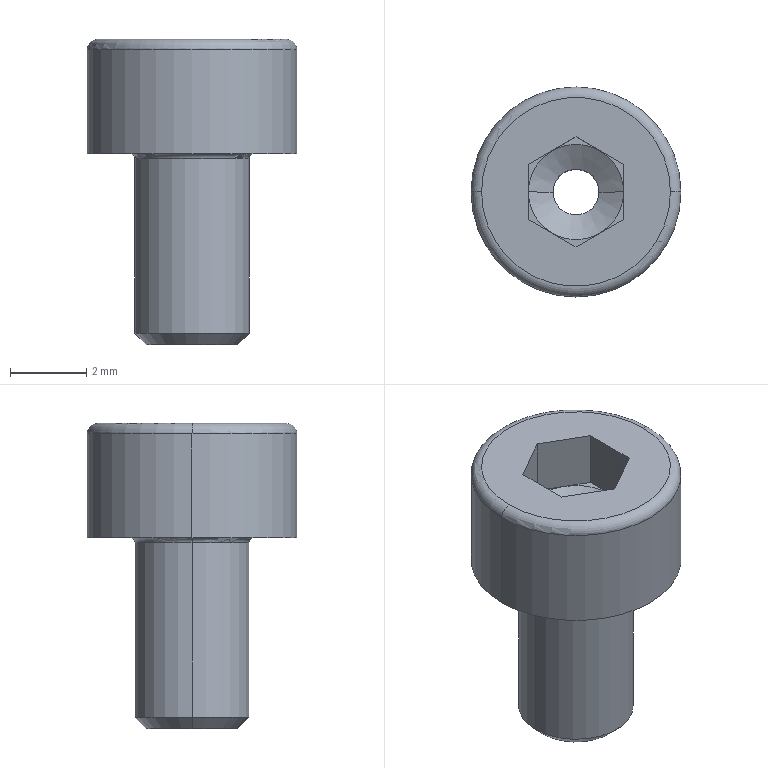Part | SolidWorks | features Fillet 2, ICE 2, Chamfer 1, Revolution 1 | 1 solid | 29 faces | box 5.5 x 5.5 x 8 mm | volume 89.884 mm3 | plane 15 | cylinder 6 | torus 4 | cone 4 | commonest cylinder face diameters 1.2 x2 3 x2 5.5 x2
STEP:
#1=CARTESIAN_POINT('',(-1.625,0.,0.));
#2=VERTEX_POINT('',#1);
#3=CARTESIAN_POINT('',(1.625,0.,0.));
#4=VERTEX_POINT('',#3);
#5=CARTESIAN_POINT('',(0.,0.,0.));
#6=DIRECTION('',(0.,0.,1.));
#7=DIRECTION('',(1.,0.,0.));
#8=AXIS2_PLACEMENT_3D('',#5,#6,#7);
#9=CIRCLE('',#8,1.625);
#10=EDGE_CURVE('',#2,#4,#9,.T.);
#11=ORIENTED_EDGE('',*,*,#10,.F.);
#12=CARTESIAN_POINT('',(-1.5,0.,-0.125));
#13=VERTEX_POINT('',#12);
#14=CARTESIAN_POINT('',(-1.625,0.,-0.125));
#15=DIRECTION('',(0.,1.,0.));
#16=DIRECTION('',(-1.,0.,0.));
#17=AXIS2_PLACEMENT_3D('',#14,#15,#16);
#18=CIRCLE('',#17,0.125);
#19=EDGE_CURVE('',#2,#13,#18,.T.);
#20=ORIENTED_EDGE('',*,*,#19,.T.);
#21=CARTESIAN_POINT('',(1.5,0.,-0.125));
#22=VERTEX_POINT('',#21);
#23=CARTESIAN_POINT('',(0.,0.,-0.125));
#24=DIRECTION('',(0.,0.,-1.));
#25=DIRECTION('',(1.,0.,0.));
#26=AXIS2_PLACEMENT_3D('',#23,#24,#25);
#27=CIRCLE('',#26,1.5);
#28=EDGE_CURVE('',#22,#13,#27,.T.);
#29=ORIENTED_EDGE('',*,*,#28,.F.);
#30=CARTESIAN_POINT('',(1.625,0.,-0.125));
#31=DIRECTION('',(0.,-1.,0.));
#32=DIRECTION('',(0.,0.,-1.));
#33=AXIS2_PLACEMENT_3D('',#30,#31,#32);
#34=CIRCLE('',#33,0.125);
#35=EDGE_CURVE('',#4,#22,#34,.T.);
#36=ORIENTED_EDGE('',*,*,#35,.F.);
#37=EDGE_LOOP('',(#11,#20,#29,#36));
#38=FACE_OUTER_BOUND('',#37,.T.);
#39=CARTESIAN_POINT('',(0.,0.,-0.125));
#40=DIRECTION('',(0.,0.,1.));
#41=DIRECTION('',(1.,0.,0.));
#42=AXIS2_PLACEMENT_3D('',#39,#40,#41);
#43=TOROIDAL_SURFACE('',#42,1.625,0.125);
#44=ADVANCED_FACE('',(#38),#43,.F.);
#45=CARTESIAN_POINT('',(-0.6,0.,1.125));
#46=VERTEX_POINT('',#45);
#47=CARTESIAN_POINT('',(0.6,0.,1.125));
#48=VERTEX_POINT('',#47);
#49=CARTESIAN_POINT('',(0.,0.,1.125));
#50=DIRECTION('',(0.,0.,1.));
#51=DIRECTION('',(1.,0.,0.));
#52=AXIS2_PLACEMENT_3D('',#49,#50,#51);
#53=CIRCLE('',#52,0.6);
#54=EDGE_CURVE('',#46,#48,#53,.T.);
#55=ORIENTED_EDGE('',*,*,#54,.F.);
#56=CARTESIAN_POINT('',(-1.25,0.,1.5));
#57=VERTEX_POINT('',#56);
#58=CARTESIAN_POINT('',(-1.25,0.,1.5));
#59=DIRECTION('',(-0.866,0.,0.5));
#60=VECTOR('',#59,1000.);
#61=LINE('',#58,#60);
#62=EDGE_CURVE('',#46,#57,#61,.T.);
#63=ORIENTED_EDGE('',*,*,#62,.T.);
#64=CARTESIAN_POINT('',(-0.625,-1.083,1.5));
#65=VERTEX_POINT('',#64);
#66=CARTESIAN_POINT('',(0.,0.,1.5));
#67=DIRECTION('',(0.,0.,1.));
#68=DIRECTION('',(1.,0.,0.));
#69=AXIS2_PLACEMENT_3D('',#66,#67,#68);
#70=CIRCLE('',#69,1.25);
#71=EDGE_CURVE('',#57,#65,#70,.T.);
#72=ORIENTED_EDGE('',*,*,#71,.T.);
#73=CARTESIAN_POINT('',(0.625,-1.083,1.5));
#74=VERTEX_POINT('',#73);
#75=CARTESIAN_POINT('',(0.,0.,1.5));
#76=DIRECTION('',(0.,0.,1.));
#77=DIRECTION('',(1.,0.,0.));
#78=AXIS2_PLACEMENT_3D('',#75,#76,#77);
#79=CIRCLE('',#78,1.25);
#80=EDGE_CURVE('',#65,#74,#79,.T.);
#81=ORIENTED_EDGE('',*,*,#80,.T.);
#82=CARTESIAN_POINT('',(1.25,0.,1.5));
#83=VERTEX_POINT('',#82);
#84=CARTESIAN_POINT('',(0.,0.,1.5));
#85=DIRECTION('',(0.,0.,1.));
#86=DIRECTION('',(1.,0.,0.));
#87=AXIS2_PLACEMENT_3D('',#84,#85,#86);
#88=CIRCLE('',#87,1.25);
#89=EDGE_CURVE('',#74,#83,#88,.T.);
#90=ORIENTED_EDGE('',*,*,#89,.T.);
#91=CARTESIAN_POINT('',(1.25,0.,1.5));
#92=DIRECTION('',(0.866,0.,0.5));
#93=VECTOR('',#92,1000.);
#94=LINE('',#91,#93);
#95=EDGE_CURVE('',#48,#83,#94,.T.);
#96=ORIENTED_EDGE('',*,*,#95,.F.);
#97=EDGE_LOOP('',(#55,#63,#72,#81,#90,#96));
#98=FACE_OUTER_BOUND('',#97,.T.);
#99=CARTESIAN_POINT('',(0.,0.,1.5));
#100=DIRECTION('',(0.,0.,1.));
#101=DIRECTION('',(1.,0.,0.));
#102=AXIS2_PLACEMENT_3D('',#99,#100,#101);
#103=CONICAL_SURFACE('',#102,1.25,1.047);
#104=ADVANCED_FACE('',(#98),#103,.F.);
#105=CARTESIAN_POINT('',(-1.2,0.,-5.));
#106=VERTEX_POINT('',#105);
#107=CARTESIAN_POINT('',(1.2,0.,-5.));
#108=VERTEX_POINT('',#107);
#109=CARTESIAN_POINT('',(0.,0.,-5.));
#110=DIRECTION('',(0.,0.,-1.));
#111=DIRECTION('',(1.,0.,0.));
#112=AXIS2_PLACEMENT_3D('',#109,#110,#111);
#113=CIRCLE('',#112,1.2);
#114=EDGE_CURVE('',#106,#108,#113,.T.);
#115=ORIENTED_EDGE('',*,*,#114,.F.);
#116=CARTESIAN_POINT('',(-1.5,0.,-4.7));
#117=VERTEX_POINT('',#116);
#118=CARTESIAN_POINT('',(-1.5,0.,-4.7));
#119=DIRECTION('',(-0.7071,0.,0.7071));
#120=VECTOR('',#119,1000.);
#121=LINE('',#118,#120);
#122=EDGE_CURVE('',#106,#117,#121,.T.);
#123=ORIENTED_EDGE('',*,*,#122,.T.);
#124=CARTESIAN_POINT('',(1.5,0.,-4.7));
#125=VERTEX_POINT('',#124);
#126=CARTESIAN_POINT('',(0.,0.,-4.7));
#127=DIRECTION('',(0.,0.,1.));
#128=DIRECTION('',(1.,0.,0.));
#129=AXIS2_PLACEMENT_3D('',#126,#127,#128);
#130=CIRCLE('',#129,1.5);
#131=EDGE_CURVE('',#125,#117,#130,.T.);
#132=ORIENTED_EDGE('',*,*,#131,.F.);
#133=CARTESIAN_POINT('',(1.5,0.,-4.7));
#134=DIRECTION('',(0.7071,0.,0.7071));
#135=VECTOR('',#134,1000.);
#136=LINE('',#133,#135);
#137=EDGE_CURVE('',#108,#125,#136,.T.);
#138=ORIENTED_EDGE('',*,*,#137,.F.);
#139=EDGE_LOOP('',(#115,#123,#132,#138));
#140=FACE_OUTER_BOUND('',#139,.T.);
#141=CARTESIAN_POINT('',(0.,0.,-4.7));
#142=DIRECTION('',(0.,0.,1.));
#143=DIRECTION('',(1.,0.,0.));
#144=AXIS2_PLACEMENT_3D('',#141,#142,#143);
#145=CONICAL_SURFACE('',#144,1.5,0.7854);
#146=ADVANCED_FACE('',(#140),#145,.T.);
#147=CARTESIAN_POINT('',(2.475,0.,3.));
#148=VERTEX_POINT('',#147);
#149=CARTESIAN_POINT('',(-2.475,0.,3.));
#150=VERTEX_POINT('',#149);
#151=CARTESIAN_POINT('',(0.,0.,3.));
#152=DIRECTION('',(0.,0.,1.));
#153=DIRECTION('',(-1.,0.,0.));
#154=AXIS2_PLACEMENT_3D('',#151,#152,#153);
#155=CIRCLE('',#154,2.475);
#156=EDGE_CURVE('',#148,#150,#155,.T.);
#157=ORIENTED_EDGE('',*,*,#156,.F.);
#158=CARTESIAN_POINT('',(2.75,0.,2.725));
#159=VERTEX_POINT('',#158);
#160=CARTESIAN_POINT('',(2.475,0.,2.725));
#161=DIRECTION('',(0.,1.,0.));
#162=DIRECTION('',(-1.,0.,0.));
#163=AXIS2_PLACEMENT_3D('',#160,#161,#162);
#164=CIRCLE('',#163,0.275);
#165=EDGE_CURVE('',#148,#159,#164,.T.);
#166=ORIENTED_EDGE('',*,*,#165,.T.);
#167=CARTESIAN_POINT('',(-2.75,0.,2.725));
#168=VERTEX_POINT('',#167);
#169=CARTESIAN_POINT('',(0.,0.,2.725));
#170=DIRECTION('',(0.,0.,-1.));
#171=DIRECTION('',(-1.,0.,0.));
#172=AXIS2_PLACEMENT_3D('',#169,#170,#171);
#173=CIRCLE('',#172,2.75);
#174=EDGE_CURVE('',#168,#159,#173,.T.);
#175=ORIENTED_EDGE('',*,*,#174,.F.);
#176=CARTESIAN_POINT('',(-2.475,0.,2.725));
#177=DIRECTION('',(0.,-1.,0.));
#178=DIRECTION('',(0.,0.,-1.));
#179=AXIS2_PLACEMENT_3D('',#176,#177,#178);
#180=CIRCLE('',#179,0.275);
#181=EDGE_CURVE('',#150,#168,#180,.T.);
#182=ORIENTED_EDGE('',*,*,#181,.F.);
#183=EDGE_LOOP('',(#157,#166,#175,#182));
#184=FACE_OUTER_BOUND('',#183,.T.);
#185=CARTESIAN_POINT('',(0.,0.,2.725));
#186=DIRECTION('',(0.,0.,-1.));
#187=DIRECTION('',(-1.,0.,0.));
#188=AXIS2_PLACEMENT_3D('',#185,#186,#187);
#189=TOROIDAL_SURFACE('',#188,2.475,0.275);
#190=ADVANCED_FACE('',(#184),#189,.T.);
#191=ORIENTED_EDGE('',*,*,#131,.T.);
#192=CARTESIAN_POINT('',(-1.5,0.,3.));
#193=DIRECTION('',(0.,0.,1.));
#194=VECTOR('',#193,1000.);
#195=LINE('',#192,#194);
#196=EDGE_CURVE('',#117,#13,#195,.T.);
#197=ORIENTED_EDGE('',*,*,#196,.T.);
#198=CARTESIAN_POINT('',(0.,0.,-0.125));
#199=DIRECTION('',(0.,0.,-1.));
#200=DIRECTION('',(1.,0.,0.));
#201=AXIS2_PLACEMENT_3D('',#198,#199,#200);
#202=CIRCLE('',#201,1.5);
#203=EDGE_CURVE('',#13,#22,#202,.T.);
#204=ORIENTED_EDGE('',*,*,#203,.T.);
#205=CARTESIAN_POINT('',(1.5,0.,3.));
#206=DIRECTION('',(0.,0.,1.));
#207=VECTOR('',#206,1000.);
#208=LINE('',#205,#207);
#209=EDGE_CURVE('',#125,#22,#208,.T.);
#210=ORIENTED_EDGE('',*,*,#209,.F.);
#211=EDGE_LOOP('',(#191,#197,#204,#210));
#212=FACE_OUTER_BOUND('',#211,.T.);
#213=CARTESIAN_POINT('',(0.,0.,3.));
#214=DIRECTION('',(0.,0.,1.));
#215=DIRECTION('',(1.,0.,0.));
#216=AXIS2_PLACEMENT_3D('',#213,#214,#215);
#217=CYLINDRICAL_SURFACE('',#216,1.5);
#218=ADVANCED_FACE('',(#212),#217,.T.);
#219=CARTESIAN_POINT('',(2.75,0.,0.));
#220=VERTEX_POINT('',#219);
#221=CARTESIAN_POINT('',(-2.75,0.,0.));
#222=VERTEX_POINT('',#221);
#223=CARTESIAN_POINT('',(0.,0.,0.));
#224=DIRECTION('',(0.,0.,1.));
#225=DIRECTION('',(1.,0.,0.));
#226=AXIS2_PLACEMENT_3D('',#223,#224,#225);
#227=CIRCLE('',#226,2.75);
#228=EDGE_CURVE('',#220,#222,#227,.T.);
#229=ORIENTED_EDGE('',*,*,#228,.T.);
#230=CARTESIAN_POINT('',(-2.75,0.,3.));
#231=DIRECTION('',(0.,0.,1.));
#232=VECTOR('',#231,1000.);
#233=LINE('',#230,#232);
#234=EDGE_CURVE('',#222,#168,#233,.T.);
#235=ORIENTED_EDGE('',*,*,#234,.T.);
#236=ORIENTED_EDGE('',*,*,#174,.T.);
#237=CARTESIAN_POINT('',(2.75,0.,3.));
#238=DIRECTION('',(0.,0.,1.));
#239=VECTOR('',#238,1000.);
#240=LINE('',#237,#239);
#241=EDGE_CURVE('',#220,#159,#240,.T.);
#242=ORIENTED_EDGE('',*,*,#241,.F.);
#243=EDGE_LOOP('',(#229,#235,#236,#242));
#244=FACE_OUTER_BOUND('',#243,.T.);
#245=CARTESIAN_POINT('',(0.,0.,3.));
#246=DIRECTION('',(0.,0.,1.));
#247=DIRECTION('',(1.,0.,0.));
#248=AXIS2_PLACEMENT_3D('',#245,#246,#247);
#249=CYLINDRICAL_SURFACE('',#248,2.75);
#250=ADVANCED_FACE('',(#244),#249,.T.);
#251=CARTESIAN_POINT('',(-0.6,0.,-5.));
#252=VERTEX_POINT('',#251);
#253=CARTESIAN_POINT('',(0.6,0.,-5.));
#254=VERTEX_POINT('',#253);
#255=CARTESIAN_POINT('',(0.,0.,-5.));
#256=DIRECTION('',(0.,0.,1.));
#257=DIRECTION('',(1.,0.,0.));
#258=AXIS2_PLACEMENT_3D('',#255,#256,#257);
#259=CIRCLE('',#258,0.6);
#260=EDGE_CURVE('',#252,#254,#259,.T.);
#261=ORIENTED_EDGE('',*,*,#260,.F.);
#262=CARTESIAN_POINT('',(-0.6,0.,3.));
#263=DIRECTION('',(0.,0.,1.));
#264=VECTOR('',#263,1000.);
#265=LINE('',#262,#264);
#266=EDGE_CURVE('',#252,#46,#265,.T.);
#267=ORIENTED_EDGE('',*,*,#266,.T.);
#268=ORIENTED_EDGE('',*,*,#54,.T.);
#269=CARTESIAN_POINT('',(0.6,0.,3.));
#270=DIRECTION('',(0.,0.,1.));
#271=VECTOR('',#270,1000.);
#272=LINE('',#269,#271);
#273=EDGE_CURVE('',#254,#48,#272,.T.);
#274=ORIENTED_EDGE('',*,*,#273,.F.);
#275=EDGE_LOOP('',(#261,#267,#268,#274));
#276=FACE_OUTER_BOUND('',#275,.T.);
#277=CARTESIAN_POINT('',(0.,0.,3.));
#278=DIRECTION('',(0.,0.,1.));
#279=DIRECTION('',(1.,0.,0.));
#280=AXIS2_PLACEMENT_3D('',#277,#278,#279);
#281=CYLINDRICAL_SURFACE('',#280,0.6);
#282=ADVANCED_FACE('',(#276),#281,.F.);
#283=CARTESIAN_POINT('',(0.625,1.083,1.5));
#284=VERTEX_POINT('',#283);
#285=CARTESIAN_POINT('',(0.,0.,1.5));
#286=DIRECTION('',(0.,0.,1.));
#287=DIRECTION('',(1.,0.,0.));
#288=AXIS2_PLACEMENT_3D('',#285,#286,#287);
#289=CIRCLE('',#288,1.25);
#290=EDGE_CURVE('',#83,#284,#289,.T.);
#291=ORIENTED_EDGE('',*,*,#290,.F.);
#292=CARTESIAN_POINT('',(1.25,0.7217,1.5));
#293=VERTEX_POINT('',#292);
#294=CARTESIAN_POINT('',(1.25,-0.7217,1.5));
#295=DIRECTION('',(0.,1.,0.));
#296=VECTOR('',#295,1000.);
#297=LINE('',#294,#296);
#298=EDGE_CURVE('',#83,#293,#297,.T.);
#299=ORIENTED_EDGE('',*,*,#298,.T.);
#300=CARTESIAN_POINT('',(1.25,0.7217,1.5));
#301=DIRECTION('',(-0.866,0.5,0.));
#302=VECTOR('',#301,1000.);
#303=LINE('',#300,#302);
#304=EDGE_CURVE('',#293,#284,#303,.T.);
#305=ORIENTED_EDGE('',*,*,#304,.T.);
#306=EDGE_LOOP('',(#291,#299,#305));
#307=FACE_OUTER_BOUND('',#306,.T.);
#308=CARTESIAN_POINT('',(0.,1.443,1.5));
#309=DIRECTION('',(0.,0.,1.));
#310=DIRECTION('',(1.,0.,0.));
#311=AXIS2_PLACEMENT_3D('',#308,#309,#310);
#312=PLANE('',#311);
#313=ADVANCED_FACE('',(#307),#312,.T.);
#314=CARTESIAN_POINT('',(-0.625,1.083,1.5));
#315=VERTEX_POINT('',#314);
#316=CARTESIAN_POINT('',(0.,0.,1.5));
#317=DIRECTION('',(0.,0.,1.));
#318=DIRECTION('',(1.,0.,0.));
#319=AXIS2_PLACEMENT_3D('',#316,#317,#318);
#320=CIRCLE('',#319,1.25);
#321=EDGE_CURVE('',#284,#315,#320,.T.);
#322=ORIENTED_EDGE('',*,*,#321,.F.);
#323=CARTESIAN_POINT('',(0.,1.443,1.5));
#324=VERTEX_POINT('',#323);
#325=CARTESIAN_POINT('',(1.25,0.7217,1.5));
#326=DIRECTION('',(-0.866,0.5,0.));
#327=VECTOR('',#326,1000.);
#328=LINE('',#325,#327);
#329=EDGE_CURVE('',#284,#324,#328,.T.);
#330=ORIENTED_EDGE('',*,*,#329,.T.);
#331=CARTESIAN_POINT('',(0.,1.443,1.5));
#332=DIRECTION('',(-0.866,-0.5,0.));
#333=VECTOR('',#332,1000.);
#334=LINE('',#331,#333);
#335=EDGE_CURVE('',#324,#315,#334,.T.);
#336=ORIENTED_EDGE('',*,*,#335,.T.);
#337=EDGE_LOOP('',(#322,#330,#336));
#338=FACE_OUTER_BOUND('',#337,.T.);
#339=CARTESIAN_POINT('',(0.,1.443,1.5));
#340=DIRECTION('',(0.,0.,1.));
#341=DIRECTION('',(1.,0.,0.));
#342=AXIS2_PLACEMENT_3D('',#339,#340,#341);
#343=PLANE('',#342);
#344=ADVANCED_FACE('',(#338),#343,.T.);
#345=CARTESIAN_POINT('',(0.,0.,1.5));
#346=DIRECTION('',(0.,0.,1.));
#347=DIRECTION('',(1.,0.,0.));
#348=AXIS2_PLACEMENT_3D('',#345,#346,#347);
#349=CIRCLE('',#348,1.25);
#350=EDGE_CURVE('',#315,#57,#349,.T.);
#351=ORIENTED_EDGE('',*,*,#350,.F.);
#352=CARTESIAN_POINT('',(-1.25,0.7217,1.5));
#353=VERTEX_POINT('',#352);
#354=CARTESIAN_POINT('',(0.,1.443,1.5));
#355=DIRECTION('',(-0.866,-0.5,0.));
#356=VECTOR('',#355,1000.);
#357=LINE('',#354,#356);
#358=EDGE_CURVE('',#315,#353,#357,.T.);
#359=ORIENTED_EDGE('',*,*,#358,.T.);
#360=CARTESIAN_POINT('',(-1.25,0.7217,1.5));
#361=DIRECTION('',(0.,-1.,0.));
#362=VECTOR('',#361,1000.);
#363=LINE('',#360,#362);
#364=EDGE_CURVE('',#353,#57,#363,.T.);
#365=ORIENTED_EDGE('',*,*,#364,.T.);
#366=EDGE_LOOP('',(#351,#359,#365));
#367=FACE_OUTER_BOUND('',#366,.T.);
#368=CARTESIAN_POINT('',(0.,1.443,1.5));
#369=DIRECTION('',(0.,0.,1.));
#370=DIRECTION('',(1.,0.,0.));
#371=AXIS2_PLACEMENT_3D('',#368,#369,#370);
#372=PLANE('',#371);
#373=ADVANCED_FACE('',(#367),#372,.T.);
#374=ORIENTED_EDGE('',*,*,#71,.F.);
#375=CARTESIAN_POINT('',(-1.25,-0.7217,1.5));
#376=VERTEX_POINT('',#375);
#377=CARTESIAN_POINT('',(-1.25,0.7217,1.5));
#378=DIRECTION('',(0.,-1.,0.));
#379=VECTOR('',#378,1000.);
#380=LINE('',#377,#379);
#381=EDGE_CURVE('',#57,#376,#380,.T.);
#382=ORIENTED_EDGE('',*,*,#381,.T.);
#383=CARTESIAN_POINT('',(-1.25,-0.7217,1.5));
#384=DIRECTION('',(0.866,-0.5,0.));
#385=VECTOR('',#384,1000.);
#386=LINE('',#383,#385);
#387=EDGE_CURVE('',#376,#65,#386,.T.);
#388=ORIENTED_EDGE('',*,*,#387,.T.);
#389=EDGE_LOOP('',(#374,#382,#388));
#390=FACE_OUTER_BOUND('',#389,.T.);
#391=CARTESIAN_POINT('',(0.,1.443,1.5));
#392=DIRECTION('',(0.,0.,1.));
#393=DIRECTION('',(1.,0.,0.));
#394=AXIS2_PLACEMENT_3D('',#391,#392,#393);
#395=PLANE('',#394);
#396=ADVANCED_FACE('',(#390),#395,.T.);
#397=ORIENTED_EDGE('',*,*,#80,.F.);
#398=CARTESIAN_POINT('',(0.,-1.443,1.5));
#399=VERTEX_POINT('',#398);
#400=CARTESIAN_POINT('',(-1.25,-0.7217,1.5));
#401=DIRECTION('',(0.866,-0.5,0.));
#402=VECTOR('',#401,1000.);
#403=LINE('',#400,#402);
#404=EDGE_CURVE('',#65,#399,#403,.T.);
#405=ORIENTED_EDGE('',*,*,#404,.T.);
#406=CARTESIAN_POINT('',(0.,-1.443,1.5));
#407=DIRECTION('',(0.866,0.5,0.));
#408=VECTOR('',#407,1000.);
#409=LINE('',#406,#408);
#410=EDGE_CURVE('',#399,#74,#409,.T.);
#411=ORIENTED_EDGE('',*,*,#410,.T.);
#412=EDGE_LOOP('',(#397,#405,#411));
#413=FACE_OUTER_BOUND('',#412,.T.);
#414=CARTESIAN_POINT('',(0.,1.443,1.5));
#415=DIRECTION('',(0.,0.,1.));
#416=DIRECTION('',(1.,0.,0.));
#417=AXIS2_PLACEMENT_3D('',#414,#415,#416);
#418=PLANE('',#417);
#419=ADVANCED_FACE('',(#413),#418,.T.);
#420=ORIENTED_EDGE('',*,*,#266,.F.);
#421=CARTESIAN_POINT('',(0.,0.,-5.));
#422=DIRECTION('',(0.,0.,1.));
#423=DIRECTION('',(1.,0.,0.));
#424=AXIS2_PLACEMENT_3D('',#421,#422,#423);
#425=CIRCLE('',#424,0.6);
#426=EDGE_CURVE('',#254,#252,#425,.T.);
#427=ORIENTED_EDGE('',*,*,#426,.F.);
#428=ORIENTED_EDGE('',*,*,#273,.T.);
#429=CARTESIAN_POINT('',(0.,0.,1.125));
#430=DIRECTION('',(0.,0.,1.));
#431=DIRECTION('',(1.,0.,0.));
#432=AXIS2_PLACEMENT_3D('',#429,#430,#431);
#433=CIRCLE('',#432,0.6);
#434=EDGE_CURVE('',#48,#46,#433,.T.);
#435=ORIENTED_EDGE('',*,*,#434,.T.);
#436=EDGE_LOOP('',(#420,#427,#428,#435));
#437=FACE_OUTER_BOUND('',#436,.T.);
#438=CARTESIAN_POINT('',(0.,0.,3.));
#439=DIRECTION('',(0.,0.,1.));
#440=DIRECTION('',(1.,0.,0.));
#441=AXIS2_PLACEMENT_3D('',#438,#439,#440);
#442=CYLINDRICAL_SURFACE('',#441,0.6);
#443=ADVANCED_FACE('',(#437),#442,.F.);
#444=ORIENTED_EDGE('',*,*,#234,.F.);
#445=CARTESIAN_POINT('',(0.,0.,0.));
#446=DIRECTION('',(0.,0.,1.));
#447=DIRECTION('',(1.,0.,0.));
#448=AXIS2_PLACEMENT_3D('',#445,#446,#447);
#449=CIRCLE('',#448,2.75);
#450=EDGE_CURVE('',#222,#220,#449,.T.);
#451=ORIENTED_EDGE('',*,*,#450,.T.);
#452=ORIENTED_EDGE('',*,*,#241,.T.);
#453=CARTESIAN_POINT('',(0.,0.,2.725));
#454=DIRECTION('',(0.,0.,-1.));
#455=DIRECTION('',(-1.,0.,0.));
#456=AXIS2_PLACEMENT_3D('',#453,#454,#455);
#457=CIRCLE('',#456,2.75);
#458=EDGE_CURVE('',#159,#168,#457,.T.);
#459=ORIENTED_EDGE('',*,*,#458,.T.);
#460=EDGE_LOOP('',(#444,#451,#452,#459));
#461=FACE_OUTER_BOUND('',#460,.T.);
#462=CARTESIAN_POINT('',(0.,0.,3.));
#463=DIRECTION('',(0.,0.,1.));
#464=DIRECTION('',(1.,0.,0.));
#465=AXIS2_PLACEMENT_3D('',#462,#463,#464);
#466=CYLINDRICAL_SURFACE('',#465,2.75);
#467=ADVANCED_FACE('',(#461),#466,.T.);
#468=CARTESIAN_POINT('',(0.,0.,0.));
#469=DIRECTION('',(0.,0.,1.));
#470=DIRECTION('',(1.,0.,0.));
#471=AXIS2_PLACEMENT_3D('',#468,#469,#470);
#472=CIRCLE('',#471,1.625);
#473=EDGE_CURVE('',#4,#2,#472,.T.);
#474=ORIENTED_EDGE('',*,*,#473,.T.);
#475=ORIENTED_EDGE('',*,*,#10,.T.);
#476=EDGE_LOOP('',(#474,#475));
#477=FACE_BOUND('',#476,.T.);
#478=ORIENTED_EDGE('',*,*,#228,.F.);
#479=ORIENTED_EDGE('',*,*,#450,.F.);
#480=EDGE_LOOP('',(#478,#479));
#481=FACE_OUTER_BOUND('',#480,.T.);
#482=CARTESIAN_POINT('',(0.,2.75,0.));
#483=DIRECTION('',(0.,0.,1.));
#484=DIRECTION('',(1.,0.,0.));
#485=AXIS2_PLACEMENT_3D('',#482,#483,#484);
#486=PLANE('',#485);
#487=ADVANCED_FACE('',(#477,#481),#486,.F.);
#488=ORIENTED_EDGE('',*,*,#196,.F.);
#489=CARTESIAN_POINT('',(0.,0.,-4.7));
#490=DIRECTION('',(0.,0.,1.));
#491=DIRECTION('',(1.,0.,0.));
#492=AXIS2_PLACEMENT_3D('',#489,#490,#491);
#493=CIRCLE('',#492,1.5);
#494=EDGE_CURVE('',#117,#125,#493,.T.);
#495=ORIENTED_EDGE('',*,*,#494,.T.);
#496=ORIENTED_EDGE('',*,*,#209,.T.);
#497=ORIENTED_EDGE('',*,*,#28,.T.);
#498=EDGE_LOOP('',(#488,#495,#496,#497));
#499=FACE_OUTER_BOUND('',#498,.T.);
#500=CARTESIAN_POINT('',(0.,0.,3.));
#501=DIRECTION('',(0.,0.,1.));
#502=DIRECTION('',(1.,0.,0.));
#503=AXIS2_PLACEMENT_3D('',#500,#501,#502);
#504=CYLINDRICAL_SURFACE('',#503,1.5);
#505=ADVANCED_FACE('',(#499),#504,.T.);
#506=CARTESIAN_POINT('',(0.,0.,-5.));
#507=DIRECTION('',(0.,0.,-1.));
#508=DIRECTION('',(1.,0.,0.));
#509=AXIS2_PLACEMENT_3D('',#506,#507,#508);
#510=CIRCLE('',#509,1.2);
#511=EDGE_CURVE('',#108,#106,#510,.T.);
#512=ORIENTED_EDGE('',*,*,#511,.T.);
#513=ORIENTED_EDGE('',*,*,#114,.T.);
#514=EDGE_LOOP('',(#512,#513));
#515=FACE_OUTER_BOUND('',#514,.T.);
#516=ORIENTED_EDGE('',*,*,#426,.T.);
#517=ORIENTED_EDGE('',*,*,#260,.T.);
#518=EDGE_LOOP('',(#516,#517));
#519=FACE_BOUND('',#518,.T.);
#520=CARTESIAN_POINT('',(0.,1.5,-5.));
#521=DIRECTION('',(0.,0.,1.));
#522=DIRECTION('',(1.,0.,0.));
#523=AXIS2_PLACEMENT_3D('',#520,#521,#522);
#524=PLANE('',#523);
#525=ADVANCED_FACE('',(#515,#519),#524,.F.);
#526=CARTESIAN_POINT('',(0.,0.,3.));
#527=DIRECTION('',(0.,0.,1.));
#528=DIRECTION('',(-1.,0.,0.));
#529=AXIS2_PLACEMENT_3D('',#526,#527,#528);
#530=CIRCLE('',#529,2.475);
#531=EDGE_CURVE('',#150,#148,#530,.T.);
#532=ORIENTED_EDGE('',*,*,#531,.T.);
#533=ORIENTED_EDGE('',*,*,#156,.T.);
#534=EDGE_LOOP('',(#532,#533));
#535=FACE_OUTER_BOUND('',#534,.T.);
#536=CARTESIAN_POINT('',(0.,1.443,3.));
#537=VERTEX_POINT('',#536);
#538=CARTESIAN_POINT('',(-1.25,0.7217,3.));
#539=VERTEX_POINT('',#538);
#540=CARTESIAN_POINT('',(0.,1.443,3.));
#541=DIRECTION('',(-0.866,-0.5,0.));
#542=VECTOR('',#541,1000.);
#543=LINE('',#540,#542);
#544=EDGE_CURVE('',#537,#539,#543,.T.);
#545=ORIENTED_EDGE('',*,*,#544,.F.);
#546=CARTESIAN_POINT('',(1.25,0.7217,3.));
#547=VERTEX_POINT('',#546);
#548=CARTESIAN_POINT('',(1.25,0.7217,3.));
#549=DIRECTION('',(-0.866,0.5,0.));
#550=VECTOR('',#549,1000.);
#551=LINE('',#548,#550);
#552=EDGE_CURVE('',#547,#537,#551,.T.);
#553=ORIENTED_EDGE('',*,*,#552,.F.);
#554=CARTESIAN_POINT('',(1.25,-0.7217,3.));
#555=VERTEX_POINT('',#554);
#556=CARTESIAN_POINT('',(1.25,-0.7217,3.));
#557=DIRECTION('',(0.,1.,0.));
#558=VECTOR('',#557,1000.);
#559=LINE('',#556,#558);
#560=EDGE_CURVE('',#555,#547,#559,.T.);
#561=ORIENTED_EDGE('',*,*,#560,.F.);
#562=CARTESIAN_POINT('',(0.,-1.443,3.));
#563=VERTEX_POINT('',#562);
#564=CARTESIAN_POINT('',(0.,-1.443,3.));
#565=DIRECTION('',(0.866,0.5,0.));
#566=VECTOR('',#565,1000.);
#567=LINE('',#564,#566);
#568=EDGE_CURVE('',#563,#555,#567,.T.);
#569=ORIENTED_EDGE('',*,*,#568,.F.);
#570=CARTESIAN_POINT('',(-1.25,-0.7217,3.));
#571=VERTEX_POINT('',#570);
#572=CARTESIAN_POINT('',(-1.25,-0.7217,3.));
#573=DIRECTION('',(0.866,-0.5,0.));
#574=VECTOR('',#573,1000.);
#575=LINE('',#572,#574);
#576=EDGE_CURVE('',#571,#563,#575,.T.);
#577=ORIENTED_EDGE('',*,*,#576,.F.);
#578=CARTESIAN_POINT('',(-1.25,0.7217,3.));
#579=DIRECTION('',(0.,-1.,0.));
#580=VECTOR('',#579,1000.);
#581=LINE('',#578,#580);
#582=EDGE_CURVE('',#539,#571,#581,.T.);
#583=ORIENTED_EDGE('',*,*,#582,.F.);
#584=EDGE_LOOP('',(#545,#553,#561,#569,#577,#583));
#585=FACE_BOUND('',#584,.T.);
#586=CARTESIAN_POINT('',(0.,0.6,3.));
#587=DIRECTION('',(0.,0.,-1.));
#588=DIRECTION('',(-1.,0.,0.));
#589=AXIS2_PLACEMENT_3D('',#586,#587,#588);
#590=PLANE('',#589);
#591=ADVANCED_FACE('',(#535,#585),#590,.F.);
#592=ORIENTED_EDGE('',*,*,#89,.F.);
#593=CARTESIAN_POINT('',(1.25,-0.7217,1.5));
#594=VERTEX_POINT('',#593);
#595=CARTESIAN_POINT('',(0.,-1.443,1.5));
#596=DIRECTION('',(0.866,0.5,0.));
#597=VECTOR('',#596,1000.);
#598=LINE('',#595,#597);
#599=EDGE_CURVE('',#74,#594,#598,.T.);
#600=ORIENTED_EDGE('',*,*,#599,.T.);
#601=CARTESIAN_POINT('',(1.25,-0.7217,1.5));
#602=DIRECTION('',(0.,1.,0.));
#603=VECTOR('',#602,1000.);
#604=LINE('',#601,#603);
#605=EDGE_CURVE('',#594,#83,#604,.T.);
#606=ORIENTED_EDGE('',*,*,#605,.T.);
#607=EDGE_LOOP('',(#592,#600,#606));
#608=FACE_OUTER_BOUND('',#607,.T.);
#609=CARTESIAN_POINT('',(0.,1.443,1.5));
#610=DIRECTION('',(0.,0.,1.));
#611=DIRECTION('',(1.,0.,0.));
#612=AXIS2_PLACEMENT_3D('',#609,#610,#611);
#613=PLANE('',#612);
#614=ADVANCED_FACE('',(#608),#613,.T.);
#615=ORIENTED_EDGE('',*,*,#552,.T.);
#616=CARTESIAN_POINT('',(0.,1.443,1.5));
#617=DIRECTION('',(0.,0.,1.));
#618=VECTOR('',#617,1000.);
#619=LINE('',#616,#618);
#620=EDGE_CURVE('',#324,#537,#619,.T.);
#621=ORIENTED_EDGE('',*,*,#620,.F.);
#622=ORIENTED_EDGE('',*,*,#329,.F.);
#623=ORIENTED_EDGE('',*,*,#304,.F.);
#624=CARTESIAN_POINT('',(1.25,0.7217,1.5));
#625=DIRECTION('',(0.,0.,1.));
#626=VECTOR('',#625,1000.);
#627=LINE('',#624,#626);
#628=EDGE_CURVE('',#293,#547,#627,.T.);
#629=ORIENTED_EDGE('',*,*,#628,.T.);
#630=EDGE_LOOP('',(#615,#621,#622,#623,#629));
#631=FACE_OUTER_BOUND('',#630,.T.);
#632=CARTESIAN_POINT('',(1.25,0.7217,1.5));
#633=DIRECTION('',(0.5,0.866,0.));
#634=DIRECTION('',(-0.866,0.5,0.));
#635=AXIS2_PLACEMENT_3D('',#632,#633,#634);
#636=PLANE('',#635);
#637=ADVANCED_FACE('',(#631),#636,.F.);
#638=ORIENTED_EDGE('',*,*,#560,.T.);
#639=ORIENTED_EDGE('',*,*,#628,.F.);
#640=ORIENTED_EDGE('',*,*,#298,.F.);
#641=ORIENTED_EDGE('',*,*,#605,.F.);
#642=CARTESIAN_POINT('',(1.25,-0.7217,1.5));
#643=DIRECTION('',(0.,0.,1.));
#644=VECTOR('',#643,1000.);
#645=LINE('',#642,#644);
#646=EDGE_CURVE('',#594,#555,#645,.T.);
#647=ORIENTED_EDGE('',*,*,#646,.T.);
#648=EDGE_LOOP('',(#638,#639,#640,#641,#647));
#649=FACE_OUTER_BOUND('',#648,.T.);
#650=CARTESIAN_POINT('',(1.25,-0.7217,1.5));
#651=DIRECTION('',(1.,0.,0.));
#652=DIRECTION('',(0.,0.,-1.));
#653=AXIS2_PLACEMENT_3D('',#650,#651,#652);
#654=PLANE('',#653);
#655=ADVANCED_FACE('',(#649),#654,.F.);
#656=ORIENTED_EDGE('',*,*,#568,.T.);
#657=ORIENTED_EDGE('',*,*,#646,.F.);
#658=ORIENTED_EDGE('',*,*,#599,.F.);
#659=ORIENTED_EDGE('',*,*,#410,.F.);
#660=CARTESIAN_POINT('',(0.,-1.443,1.5));
#661=DIRECTION('',(0.,0.,1.));
#662=VECTOR('',#661,1000.);
#663=LINE('',#660,#662);
#664=EDGE_CURVE('',#399,#563,#663,.T.);
#665=ORIENTED_EDGE('',*,*,#664,.T.);
#666=EDGE_LOOP('',(#656,#657,#658,#659,#665));
#667=FACE_OUTER_BOUND('',#666,.T.);
#668=CARTESIAN_POINT('',(0.,-1.443,1.5));
#669=DIRECTION('',(0.5,-0.866,0.));
#670=DIRECTION('',(0.866,0.5,0.));
#671=AXIS2_PLACEMENT_3D('',#668,#669,#670);
#672=PLANE('',#671);
#673=ADVANCED_FACE('',(#667),#672,.F.);
#674=ORIENTED_EDGE('',*,*,#576,.T.);
#675=ORIENTED_EDGE('',*,*,#664,.F.);
#676=ORIENTED_EDGE('',*,*,#404,.F.);
#677=ORIENTED_EDGE('',*,*,#387,.F.);
#678=CARTESIAN_POINT('',(-1.25,-0.7217,1.5));
#679=DIRECTION('',(0.,0.,1.));
#680=VECTOR('',#679,1000.);
#681=LINE('',#678,#680);
#682=EDGE_CURVE('',#376,#571,#681,.T.);
#683=ORIENTED_EDGE('',*,*,#682,.T.);
#684=EDGE_LOOP('',(#674,#675,#676,#677,#683));
#685=FACE_OUTER_BOUND('',#684,.T.);
#686=CARTESIAN_POINT('',(-1.25,-0.7217,1.5));
#687=DIRECTION('',(-0.5,-0.866,0.));
#688=DIRECTION('',(0.866,-0.5,0.));
#689=AXIS2_PLACEMENT_3D('',#686,#687,#688);
#690=PLANE('',#689);
#691=ADVANCED_FACE('',(#685),#690,.F.);
#692=ORIENTED_EDGE('',*,*,#582,.T.);
#693=ORIENTED_EDGE('',*,*,#682,.F.);
#694=ORIENTED_EDGE('',*,*,#381,.F.);
#695=ORIENTED_EDGE('',*,*,#364,.F.);
#696=CARTESIAN_POINT('',(-1.25,0.7217,1.5));
#697=DIRECTION('',(0.,0.,1.));
#698=VECTOR('',#697,1000.);
#699=LINE('',#696,#698);
#700=EDGE_CURVE('',#353,#539,#699,.T.);
#701=ORIENTED_EDGE('',*,*,#700,.T.);
#702=EDGE_LOOP('',(#692,#693,#694,#695,#701));
#703=FACE_OUTER_BOUND('',#702,.T.);
#704=CARTESIAN_POINT('',(-1.25,0.7217,1.5));
#705=DIRECTION('',(-1.,0.,0.));
#706=DIRECTION('',(0.,-1.,0.));
#707=AXIS2_PLACEMENT_3D('',#704,#705,#706);
#708=PLANE('',#707);
#709=ADVANCED_FACE('',(#703),#708,.F.);
#710=ORIENTED_EDGE('',*,*,#544,.T.);
#711=ORIENTED_EDGE('',*,*,#700,.F.);
#712=ORIENTED_EDGE('',*,*,#358,.F.);
#713=ORIENTED_EDGE('',*,*,#335,.F.);
#714=ORIENTED_EDGE('',*,*,#620,.T.);
#715=EDGE_LOOP('',(#710,#711,#712,#713,#714));
#716=FACE_OUTER_BOUND('',#715,.T.);
#717=CARTESIAN_POINT('',(0.,1.443,1.5));
#718=DIRECTION('',(-0.5,0.866,0.));
#719=DIRECTION('',(-0.866,-0.5,0.));
#720=AXIS2_PLACEMENT_3D('',#717,#718,#719);
#721=PLANE('',#720);
#722=ADVANCED_FACE('',(#716),#721,.F.);
#723=ORIENTED_EDGE('',*,*,#165,.F.);
#724=ORIENTED_EDGE('',*,*,#531,.F.);
#725=ORIENTED_EDGE('',*,*,#181,.T.);
#726=ORIENTED_EDGE('',*,*,#458,.F.);
#727=EDGE_LOOP('',(#723,#724,#725,#726));
#728=FACE_OUTER_BOUND('',#727,.T.);
#729=CARTESIAN_POINT('',(0.,0.,2.725));
#730=DIRECTION('',(0.,0.,-1.));
#731=DIRECTION('',(-1.,0.,0.));
#732=AXIS2_PLACEMENT_3D('',#729,#730,#731);
#733=TOROIDAL_SURFACE('',#732,2.475,0.275);
#734=ADVANCED_FACE('',(#728),#733,.T.);
#735=ORIENTED_EDGE('',*,*,#122,.F.);
#736=ORIENTED_EDGE('',*,*,#511,.F.);
#737=ORIENTED_EDGE('',*,*,#137,.T.);
#738=ORIENTED_EDGE('',*,*,#494,.F.);
#739=EDGE_LOOP('',(#735,#736,#737,#738));
#740=FACE_OUTER_BOUND('',#739,.T.);
#741=CARTESIAN_POINT('',(0.,0.,-4.7));
#742=DIRECTION('',(0.,0.,1.));
#743=DIRECTION('',(1.,0.,0.));
#744=AXIS2_PLACEMENT_3D('',#741,#742,#743);
#745=CONICAL_SURFACE('',#744,1.5,0.7854);
#746=ADVANCED_FACE('',(#740),#745,.T.);
#747=ORIENTED_EDGE('',*,*,#62,.F.);
#748=ORIENTED_EDGE('',*,*,#434,.F.);
#749=ORIENTED_EDGE('',*,*,#95,.T.);
#750=ORIENTED_EDGE('',*,*,#290,.T.);
#751=ORIENTED_EDGE('',*,*,#321,.T.);
#752=ORIENTED_EDGE('',*,*,#350,.T.);
#753=EDGE_LOOP('',(#747,#748,#749,#750,#751,#752));
#754=FACE_OUTER_BOUND('',#753,.T.);
#755=CARTESIAN_POINT('',(0.,0.,1.5));
#756=DIRECTION('',(0.,0.,1.));
#757=DIRECTION('',(1.,0.,0.));
#758=AXIS2_PLACEMENT_3D('',#755,#756,#757);
#759=CONICAL_SURFACE('',#758,1.25,1.047);
#760=ADVANCED_FACE('',(#754),#759,.F.);
#761=ORIENTED_EDGE('',*,*,#19,.F.);
#762=ORIENTED_EDGE('',*,*,#473,.F.);
#763=ORIENTED_EDGE('',*,*,#35,.T.);
#764=ORIENTED_EDGE('',*,*,#203,.F.);
#765=EDGE_LOOP('',(#761,#762,#763,#764));
#766=FACE_OUTER_BOUND('',#765,.T.);
#767=CARTESIAN_POINT('',(0.,0.,-0.125));
#768=DIRECTION('',(0.,0.,1.));
#769=DIRECTION('',(1.,0.,0.));
#770=AXIS2_PLACEMENT_3D('',#767,#768,#769);
#771=TOROIDAL_SURFACE('',#770,1.625,0.125);
#772=ADVANCED_FACE('',(#766),#771,.F.);
#773=CLOSED_SHELL('',(#44,#104,#146,#190,#218,#250,#282,#313,#344,#373,#396,#419,#443,#467,#487,#505,#525,#591,#614,#637,#655,#673,#691,#709,#722,#734,#746,#760,#772));
#774=MANIFOLD_SOLID_BREP('',#773);
#775=CARTESIAN_POINT('',(0.,0.,0.));
#776=DIRECTION('',(0.,0.,1.));
#777=DIRECTION('',(1.,0.,0.));
#778=AXIS2_PLACEMENT_3D('',#775,#776,#777);
#779=(LENGTH_UNIT()NAMED_UNIT(*)SI_UNIT(.MILLI.,.METRE.));
#780=UNCERTAINTY_MEASURE_WITH_UNIT(LENGTH_MEASURE(0.00001),#779,'','');
#781=(NAMED_UNIT(*)PLANE_ANGLE_UNIT()SI_UNIT($,.RADIAN.));
#782=(NAMED_UNIT(*)SI_UNIT($,.STERADIAN.)SOLID_ANGLE_UNIT());
#783=(GEOMETRIC_REPRESENTATION_CONTEXT(3)GLOBAL_UNCERTAINTY_ASSIGNED_CONTEXT((#780))GLOBAL_UNIT_ASSIGNED_CONTEXT((#779,#781,#782))REPRESENTATION_CONTEXT('',''));
#784=ADVANCED_BREP_SHAPE_REPRESENTATION('',(#774,#778),#783);